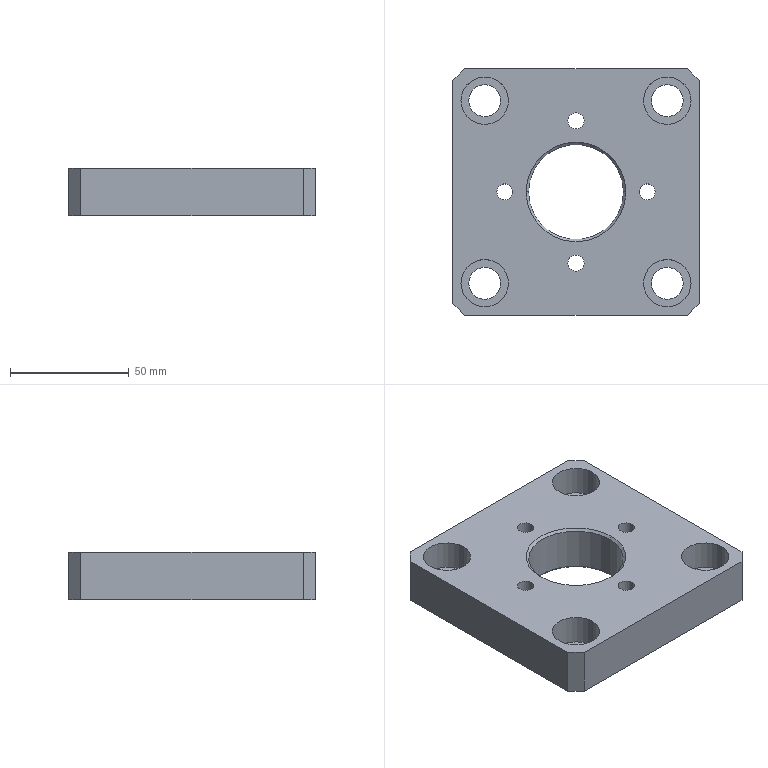Part | STEP file | Clamping Cylinder Mounting Plate | 1 solid | 44 faces | box 104 x 104 x 20 mm | volume 167084 mm3 | cylinder 26 | plane 14 | cone 4 | commonest cylinder face diameters 6.8 x8 13.5 x8 20 x8 40 x2